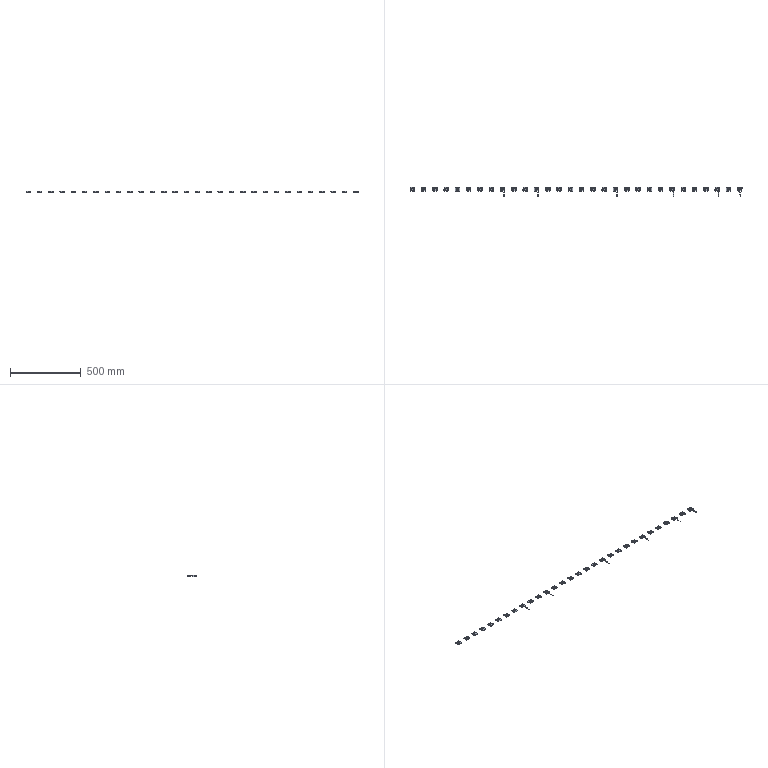Part | NX | 96 solids | 2832 faces | box 2352 x 68.4 x 12 mm | volume 173075 mm3 | plane 2148 | cylinder 624 | cone 60 | commonest cylinder face diameters 3.5 x180 2.5 x120 4 x120 6 x120 1 x60 2.1 x12